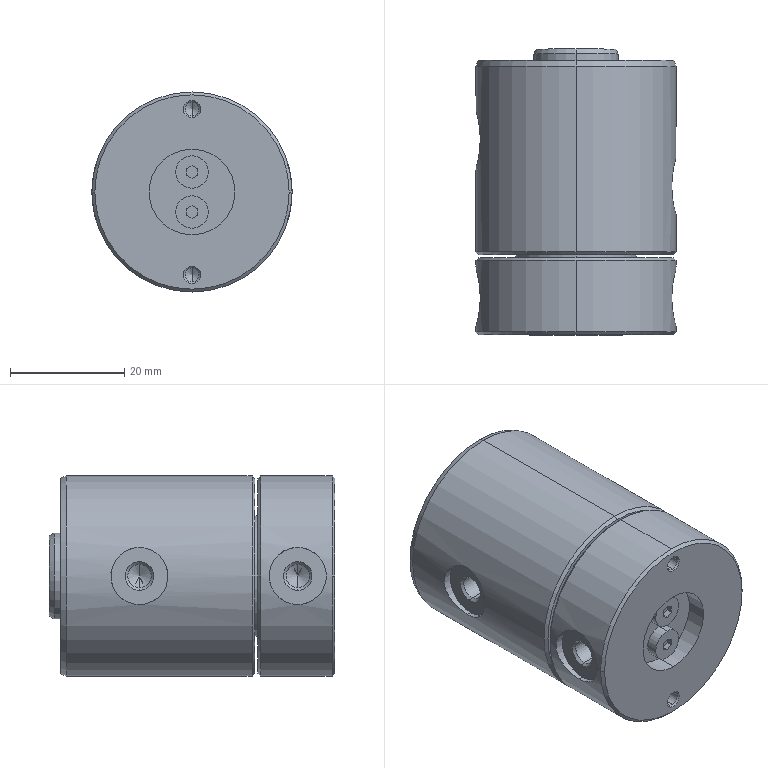Part | SolidWorks | features BaseBody 2 | 2 solids | 118 faces | box 35 x 50 x 35 mm | volume 44725 mm3 | cone 46 | cylinder 44 | plane 28 | commonest cylinder face diameters 2.459 x8 4.134 x8 10 x8 15 x6 5.7 x4 35 x4